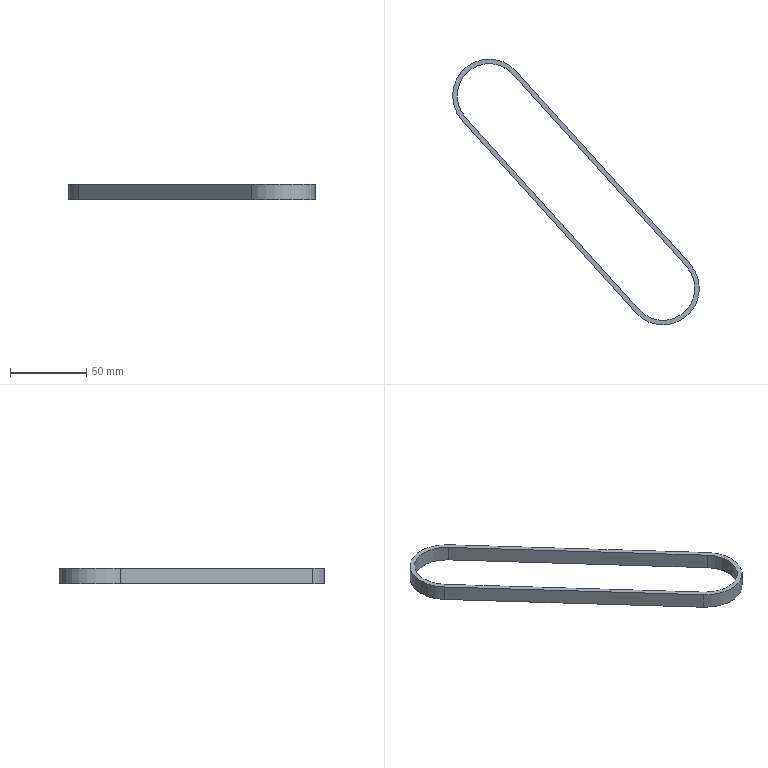Part | STEP file | 1 solid | 12 faces | box 161.812 x 174.281 x 10 mm | volume 14441 mm3 | plane 6 | cylinder 6 | commonest cylinder face diameters 42 x3 48 x3
STEP:
#1=CARTESIAN_POINT('',(0.,0.,0.));
#2=DIRECTION('',(0.,0.,1.));
#3=DIRECTION('',(1.,0.,0.));
#4=AXIS2_PLACEMENT_3D('',#1,#2,#3);
#5=CARTESIAN_POINT('',(15.599,14.059,-2.));
#6=VERTEX_POINT('',#5);
#7=CARTESIAN_POINT('',(-98.213,140.34,-2.));
#8=VERTEX_POINT('',#7);
#9=CARTESIAN_POINT('',(15.599,14.059,-2.));
#10=DIRECTION('',(-0.6695,0.7428,0.));
#11=VECTOR('',#10,1.);
#12=LINE('',#9,#11);
#13=CARTESIAN_POINT('',(15.599,14.059,-12.));
#14=DIRECTION('',(0.7428,0.6695,0.));
#15=DIRECTION('',(0.,0.,-1.));
#16=AXIS2_PLACEMENT_3D('',#13,#14,#15);
#17=PLANE('',#16);
#18=CARTESIAN_POINT('',(-10.,0.));
#19=DIRECTION('',(0.,1.));
#20=VECTOR('',#19,1.);
#21=LINE('',#18,#20);
#22=(GEOMETRIC_REPRESENTATION_CONTEXT(2)PARAMETRIC_REPRESENTATION_CONTEXT()REPRESENTATION_CONTEXT('',''));
#23=DEFINITIONAL_REPRESENTATION('',(#21),#22);
#24=PCURVE('',#17,#23);
#25=CARTESIAN_POINT('',(0.,0.,-2.));
#26=DIRECTION('',(0.,0.,1.));
#27=DIRECTION('',(1.,0.,0.));
#28=AXIS2_PLACEMENT_3D('',#25,#26,#27);
#29=PLANE('',#28);
#30=CARTESIAN_POINT('',(15.599,14.059));
#31=DIRECTION('',(-0.6695,0.7428));
#32=VECTOR('',#31,1.);
#33=LINE('',#30,#32);
#34=(GEOMETRIC_REPRESENTATION_CONTEXT(2)PARAMETRIC_REPRESENTATION_CONTEXT()REPRESENTATION_CONTEXT('',''));
#35=DEFINITIONAL_REPRESENTATION('',(#33),#34);
#36=PCURVE('',#29,#35);
#37=SURFACE_CURVE('',#12,(#24,#36),.PCURVE_S1.);
#38=EDGE_CURVE('',#6,#8,#37,.T.);
#39=ORIENTED_EDGE('',*,*,#38,.T.);
#40=CARTESIAN_POINT('',(-98.213,140.34,-12.));
#41=VERTEX_POINT('',#40);
#42=CARTESIAN_POINT('',(-98.213,140.34,-12.));
#43=DIRECTION('',(0.,0.,1.));
#44=VECTOR('',#43,1.);
#45=LINE('',#42,#44);
#46=CARTESIAN_POINT('',(0.,170.));
#47=DIRECTION('',(-1.,0.));
#48=VECTOR('',#47,1.);
#49=LINE('',#46,#48);
#50=(GEOMETRIC_REPRESENTATION_CONTEXT(2)PARAMETRIC_REPRESENTATION_CONTEXT()REPRESENTATION_CONTEXT('',''));
#51=DEFINITIONAL_REPRESENTATION('',(#49),#50);
#52=PCURVE('',#17,#51);
#53=CARTESIAN_POINT('',(-113.812,126.281,-12.));
#54=DIRECTION('',(0.,0.,1.));
#55=DIRECTION('',(1.,0.,0.));
#56=AXIS2_PLACEMENT_3D('',#53,#54,#55);
#57=CYLINDRICAL_SURFACE('',#56,21.);
#58=CARTESIAN_POINT('',(0.7335,0.));
#59=DIRECTION('',(0.,1.));
#60=VECTOR('',#59,1.);
#61=LINE('',#58,#60);
#62=(GEOMETRIC_REPRESENTATION_CONTEXT(2)PARAMETRIC_REPRESENTATION_CONTEXT()REPRESENTATION_CONTEXT('',''));
#63=DEFINITIONAL_REPRESENTATION('',(#61),#62);
#64=PCURVE('',#57,#63);
#65=SURFACE_CURVE('',#45,(#52,#64),.PCURVE_S1.);
#66=EDGE_CURVE('',#41,#8,#65,.T.);
#67=ORIENTED_EDGE('',*,*,#66,.F.);
#68=CARTESIAN_POINT('',(15.599,14.059,-12.));
#69=VERTEX_POINT('',#68);
#70=CARTESIAN_POINT('',(15.599,14.059,-12.));
#71=DIRECTION('',(-0.6695,0.7428,0.));
#72=VECTOR('',#71,1.);
#73=LINE('',#70,#72);
#74=CARTESIAN_POINT('',(0.,0.));
#75=DIRECTION('',(0.,1.));
#76=VECTOR('',#75,1.);
#77=LINE('',#74,#76);
#78=(GEOMETRIC_REPRESENTATION_CONTEXT(2)PARAMETRIC_REPRESENTATION_CONTEXT()REPRESENTATION_CONTEXT('',''));
#79=DEFINITIONAL_REPRESENTATION('',(#77),#78);
#80=PCURVE('',#17,#79);
#81=CARTESIAN_POINT('',(0.,0.,-12.));
#82=DIRECTION('',(0.,0.,1.));
#83=DIRECTION('',(1.,0.,0.));
#84=AXIS2_PLACEMENT_3D('',#81,#82,#83);
#85=PLANE('',#84);
#86=CARTESIAN_POINT('',(15.599,14.059));
#87=DIRECTION('',(-0.6695,0.7428));
#88=VECTOR('',#87,1.);
#89=LINE('',#86,#88);
#90=(GEOMETRIC_REPRESENTATION_CONTEXT(2)PARAMETRIC_REPRESENTATION_CONTEXT()REPRESENTATION_CONTEXT('',''));
#91=DEFINITIONAL_REPRESENTATION('',(#89),#90);
#92=PCURVE('',#85,#91);
#93=SURFACE_CURVE('',#73,(#80,#92),.PCURVE_S1.);
#94=EDGE_CURVE('',#69,#41,#93,.T.);
#95=ORIENTED_EDGE('',*,*,#94,.F.);
#96=CARTESIAN_POINT('',(15.599,14.059,-12.));
#97=DIRECTION('',(0.,0.,1.));
#98=VECTOR('',#97,1.);
#99=LINE('',#96,#98);
#100=CARTESIAN_POINT('',(0.,0.));
#101=DIRECTION('',(-1.,0.));
#102=VECTOR('',#101,1.);
#103=LINE('',#100,#102);
#104=(GEOMETRIC_REPRESENTATION_CONTEXT(2)PARAMETRIC_REPRESENTATION_CONTEXT()REPRESENTATION_CONTEXT('',''));
#105=DEFINITIONAL_REPRESENTATION('',(#103),#104);
#106=PCURVE('',#17,#105);
#107=CARTESIAN_POINT('',(0.,0.,-12.));
#108=DIRECTION('',(0.,0.,1.));
#109=DIRECTION('',(1.,0.,0.));
#110=AXIS2_PLACEMENT_3D('',#107,#108,#109);
#111=CYLINDRICAL_SURFACE('',#110,21.);
#112=CARTESIAN_POINT('',(0.7335,0.));
#113=DIRECTION('',(0.,1.));
#114=VECTOR('',#113,1.);
#115=LINE('',#112,#114);
#116=(GEOMETRIC_REPRESENTATION_CONTEXT(2)PARAMETRIC_REPRESENTATION_CONTEXT()REPRESENTATION_CONTEXT('',''));
#117=DEFINITIONAL_REPRESENTATION('',(#115),#116);
#118=PCURVE('',#111,#117);
#119=SURFACE_CURVE('',#99,(#106,#118),.PCURVE_S1.);
#120=EDGE_CURVE('',#69,#6,#119,.T.);
#121=ORIENTED_EDGE('',*,*,#120,.T.);
#122=EDGE_LOOP('',(#39,#67,#95,#121));
#123=FACE_BOUND('',#122,.T.);
#124=ADVANCED_FACE('',(#123),#17,.F.);
#125=ORIENTED_EDGE('',*,*,#66,.F.);
#126=CARTESIAN_POINT('',(-129.411,112.222,-12.));
#127=VERTEX_POINT('',#126);
#128=CARTESIAN_POINT('',(-113.812,126.281,-12.));
#129=DIRECTION('',(0.,0.,1.));
#130=DIRECTION('',(1.,0.,0.));
#131=AXIS2_PLACEMENT_3D('',#128,#129,#130);
#132=CIRCLE('',#131,21.);
#133=CARTESIAN_POINT('',(0.,0.));
#134=DIRECTION('',(1.,0.));
#135=VECTOR('',#134,1.);
#136=LINE('',#133,#135);
#137=(GEOMETRIC_REPRESENTATION_CONTEXT(2)PARAMETRIC_REPRESENTATION_CONTEXT()REPRESENTATION_CONTEXT('',''));
#138=DEFINITIONAL_REPRESENTATION('',(#136),#137);
#139=PCURVE('',#57,#138);
#140=CARTESIAN_POINT('',(-113.812,126.281));
#141=DIRECTION('',(1.,0.));
#142=AXIS2_PLACEMENT_2D('',#140,#141);
#143=CIRCLE('',#142,21.);
#144=(GEOMETRIC_REPRESENTATION_CONTEXT(2)PARAMETRIC_REPRESENTATION_CONTEXT()REPRESENTATION_CONTEXT('',''));
#145=DEFINITIONAL_REPRESENTATION('',(#143),#144);
#146=PCURVE('',#85,#145);
#147=SURFACE_CURVE('',#132,(#139,#146),.PCURVE_S1.);
#148=EDGE_CURVE('',#41,#127,#147,.T.);
#149=ORIENTED_EDGE('',*,*,#148,.T.);
#150=CARTESIAN_POINT('',(-129.411,112.222,-2.));
#151=VERTEX_POINT('',#150);
#152=CARTESIAN_POINT('',(-129.411,112.222,-12.));
#153=DIRECTION('',(0.,0.,1.));
#154=VECTOR('',#153,1.);
#155=LINE('',#152,#154);
#156=CARTESIAN_POINT('',(3.875,0.));
#157=DIRECTION('',(0.,1.));
#158=VECTOR('',#157,1.);
#159=LINE('',#156,#158);
#160=(GEOMETRIC_REPRESENTATION_CONTEXT(2)PARAMETRIC_REPRESENTATION_CONTEXT()REPRESENTATION_CONTEXT('',''));
#161=DEFINITIONAL_REPRESENTATION('',(#159),#160);
#162=PCURVE('',#57,#161);
#163=CARTESIAN_POINT('',(-15.599,-14.059,-12.));
#164=DIRECTION('',(-0.7428,-0.6695,0.));
#165=DIRECTION('',(-0.6695,0.7428,0.));
#166=AXIS2_PLACEMENT_3D('',#163,#164,#165);
#167=PLANE('',#166);
#168=CARTESIAN_POINT('',(170.,0.));
#169=DIRECTION('',(0.,-1.));
#170=VECTOR('',#169,1.);
#171=LINE('',#168,#170);
#172=(GEOMETRIC_REPRESENTATION_CONTEXT(2)PARAMETRIC_REPRESENTATION_CONTEXT()REPRESENTATION_CONTEXT('',''));
#173=DEFINITIONAL_REPRESENTATION('',(#171),#172);
#174=PCURVE('',#167,#173);
#175=SURFACE_CURVE('',#155,(#162,#174),.PCURVE_S1.);
#176=EDGE_CURVE('',#127,#151,#175,.T.);
#177=ORIENTED_EDGE('',*,*,#176,.T.);
#178=CARTESIAN_POINT('',(-113.812,126.281,-2.));
#179=DIRECTION('',(0.,0.,1.));
#180=DIRECTION('',(1.,0.,0.));
#181=AXIS2_PLACEMENT_3D('',#178,#179,#180);
#182=CIRCLE('',#181,21.);
#183=CARTESIAN_POINT('',(0.,10.));
#184=DIRECTION('',(1.,0.));
#185=VECTOR('',#184,1.);
#186=LINE('',#183,#185);
#187=(GEOMETRIC_REPRESENTATION_CONTEXT(2)PARAMETRIC_REPRESENTATION_CONTEXT()REPRESENTATION_CONTEXT('',''));
#188=DEFINITIONAL_REPRESENTATION('',(#186),#187);
#189=PCURVE('',#57,#188);
#190=CARTESIAN_POINT('',(-113.812,126.281));
#191=DIRECTION('',(1.,0.));
#192=AXIS2_PLACEMENT_2D('',#190,#191);
#193=CIRCLE('',#192,21.);
#194=(GEOMETRIC_REPRESENTATION_CONTEXT(2)PARAMETRIC_REPRESENTATION_CONTEXT()REPRESENTATION_CONTEXT('',''));
#195=DEFINITIONAL_REPRESENTATION('',(#193),#194);
#196=PCURVE('',#29,#195);
#197=SURFACE_CURVE('',#182,(#189,#196),.PCURVE_S1.);
#198=EDGE_CURVE('',#8,#151,#197,.T.);
#199=ORIENTED_EDGE('',*,*,#198,.F.);
#200=EDGE_LOOP('',(#125,#149,#177,#199));
#201=FACE_BOUND('',#200,.F.);
#202=ADVANCED_FACE('',(#201),#57,.F.);
#203=CARTESIAN_POINT('',(-15.599,-14.059,-2.));
#204=VERTEX_POINT('',#203);
#205=CARTESIAN_POINT('',(-15.599,-14.059,-2.));
#206=DIRECTION('',(0.6695,-0.7428,0.));
#207=VECTOR('',#206,1.);
#208=LINE('',#205,#207);
#209=CARTESIAN_POINT('',(0.,-10.));
#210=DIRECTION('',(-1.,0.));
#211=VECTOR('',#210,1.);
#212=LINE('',#209,#211);
#213=(GEOMETRIC_REPRESENTATION_CONTEXT(2)PARAMETRIC_REPRESENTATION_CONTEXT()REPRESENTATION_CONTEXT('',''));
#214=DEFINITIONAL_REPRESENTATION('',(#212),#213);
#215=PCURVE('',#167,#214);
#216=CARTESIAN_POINT('',(-15.599,-14.059));
#217=DIRECTION('',(0.6695,-0.7428));
#218=VECTOR('',#217,1.);
#219=LINE('',#216,#218);
#220=(GEOMETRIC_REPRESENTATION_CONTEXT(2)PARAMETRIC_REPRESENTATION_CONTEXT()REPRESENTATION_CONTEXT('',''));
#221=DEFINITIONAL_REPRESENTATION('',(#219),#220);
#222=PCURVE('',#29,#221);
#223=SURFACE_CURVE('',#208,(#215,#222),.PCURVE_S1.);
#224=EDGE_CURVE('',#151,#204,#223,.T.);
#225=ORIENTED_EDGE('',*,*,#224,.T.);
#226=CARTESIAN_POINT('',(-15.599,-14.059,-12.));
#227=VERTEX_POINT('',#226);
#228=CARTESIAN_POINT('',(-15.599,-14.059,-12.));
#229=DIRECTION('',(0.,0.,1.));
#230=VECTOR('',#229,1.);
#231=LINE('',#228,#230);
#232=CARTESIAN_POINT('',(0.,0.));
#233=DIRECTION('',(0.,-1.));
#234=VECTOR('',#233,1.);
#235=LINE('',#232,#234);
#236=(GEOMETRIC_REPRESENTATION_CONTEXT(2)PARAMETRIC_REPRESENTATION_CONTEXT()REPRESENTATION_CONTEXT('',''));
#237=DEFINITIONAL_REPRESENTATION('',(#235),#236);
#238=PCURVE('',#167,#237);
#239=CARTESIAN_POINT('',(0.,0.,-12.));
#240=DIRECTION('',(0.,0.,1.));
#241=DIRECTION('',(1.,0.,0.));
#242=AXIS2_PLACEMENT_3D('',#239,#240,#241);
#243=CYLINDRICAL_SURFACE('',#242,21.);
#244=CARTESIAN_POINT('',(3.875,0.));
#245=DIRECTION('',(0.,1.));
#246=VECTOR('',#245,1.);
#247=LINE('',#244,#246);
#248=(GEOMETRIC_REPRESENTATION_CONTEXT(2)PARAMETRIC_REPRESENTATION_CONTEXT()REPRESENTATION_CONTEXT('',''));
#249=DEFINITIONAL_REPRESENTATION('',(#247),#248);
#250=PCURVE('',#243,#249);
#251=SURFACE_CURVE('',#231,(#238,#250),.PCURVE_S1.);
#252=EDGE_CURVE('',#227,#204,#251,.T.);
#253=ORIENTED_EDGE('',*,*,#252,.F.);
#254=CARTESIAN_POINT('',(-15.599,-14.059,-12.));
#255=DIRECTION('',(0.6695,-0.7428,0.));
#256=VECTOR('',#255,1.);
#257=LINE('',#254,#256);
#258=CARTESIAN_POINT('',(0.,0.));
#259=DIRECTION('',(-1.,0.));
#260=VECTOR('',#259,1.);
#261=LINE('',#258,#260);
#262=(GEOMETRIC_REPRESENTATION_CONTEXT(2)PARAMETRIC_REPRESENTATION_CONTEXT()REPRESENTATION_CONTEXT('',''));
#263=DEFINITIONAL_REPRESENTATION('',(#261),#262);
#264=PCURVE('',#167,#263);
#265=CARTESIAN_POINT('',(-15.599,-14.059));
#266=DIRECTION('',(0.6695,-0.7428));
#267=VECTOR('',#266,1.);
#268=LINE('',#265,#267);
#269=(GEOMETRIC_REPRESENTATION_CONTEXT(2)PARAMETRIC_REPRESENTATION_CONTEXT()REPRESENTATION_CONTEXT('',''));
#270=DEFINITIONAL_REPRESENTATION('',(#268),#269);
#271=PCURVE('',#85,#270);
#272=SURFACE_CURVE('',#257,(#264,#271),.PCURVE_S1.);
#273=EDGE_CURVE('',#127,#227,#272,.T.);
#274=ORIENTED_EDGE('',*,*,#273,.F.);
#275=ORIENTED_EDGE('',*,*,#176,.T.);
#276=EDGE_LOOP('',(#225,#253,#274,#275));
#277=FACE_BOUND('',#276,.T.);
#278=ADVANCED_FACE('',(#277),#167,.F.);
#279=CARTESIAN_POINT('',(21.,0.,-2.));
#280=VERTEX_POINT('',#279);
#281=CARTESIAN_POINT('',(0.,0.,-2.));
#282=DIRECTION('',(0.,0.,1.));
#283=DIRECTION('',(1.,0.,0.));
#284=AXIS2_PLACEMENT_3D('',#281,#282,#283);
#285=CIRCLE('',#284,21.);
#286=CARTESIAN_POINT('',(0.,10.));
#287=DIRECTION('',(1.,0.));
#288=VECTOR('',#287,1.);
#289=LINE('',#286,#288);
#290=(GEOMETRIC_REPRESENTATION_CONTEXT(2)PARAMETRIC_REPRESENTATION_CONTEXT()REPRESENTATION_CONTEXT('',''));
#291=DEFINITIONAL_REPRESENTATION('',(#289),#290);
#292=PCURVE('',#243,#291);
#293=CARTESIAN_POINT('',(0.,0.));
#294=DIRECTION('',(1.,0.));
#295=AXIS2_PLACEMENT_2D('',#293,#294);
#296=CIRCLE('',#295,21.);
#297=(GEOMETRIC_REPRESENTATION_CONTEXT(2)PARAMETRIC_REPRESENTATION_CONTEXT()REPRESENTATION_CONTEXT('',''));
#298=DEFINITIONAL_REPRESENTATION('',(#296),#297);
#299=PCURVE('',#29,#298);
#300=SURFACE_CURVE('',#285,(#292,#299),.PCURVE_S1.);
#301=EDGE_CURVE('',#204,#280,#300,.T.);
#302=ORIENTED_EDGE('',*,*,#301,.F.);
#303=ORIENTED_EDGE('',*,*,#252,.F.);
#304=CARTESIAN_POINT('',(21.,0.,-12.));
#305=VERTEX_POINT('',#304);
#306=CARTESIAN_POINT('',(0.,0.,-12.));
#307=DIRECTION('',(0.,0.,1.));
#308=DIRECTION('',(1.,0.,0.));
#309=AXIS2_PLACEMENT_3D('',#306,#307,#308);
#310=CIRCLE('',#309,21.);
#311=CARTESIAN_POINT('',(0.,0.));
#312=DIRECTION('',(1.,0.));
#313=VECTOR('',#312,1.);
#314=LINE('',#311,#313);
#315=(GEOMETRIC_REPRESENTATION_CONTEXT(2)PARAMETRIC_REPRESENTATION_CONTEXT()REPRESENTATION_CONTEXT('',''));
#316=DEFINITIONAL_REPRESENTATION('',(#314),#315);
#317=PCURVE('',#243,#316);
#318=CARTESIAN_POINT('',(0.,0.));
#319=DIRECTION('',(1.,0.));
#320=AXIS2_PLACEMENT_2D('',#318,#319);
#321=CIRCLE('',#320,21.);
#322=(GEOMETRIC_REPRESENTATION_CONTEXT(2)PARAMETRIC_REPRESENTATION_CONTEXT()REPRESENTATION_CONTEXT('',''));
#323=DEFINITIONAL_REPRESENTATION('',(#321),#322);
#324=PCURVE('',#85,#323);
#325=SURFACE_CURVE('',#310,(#317,#324),.PCURVE_S1.);
#326=EDGE_CURVE('',#227,#305,#325,.T.);
#327=ORIENTED_EDGE('',*,*,#326,.T.);
#328=CARTESIAN_POINT('',(21.,0.,-12.));
#329=DIRECTION('',(0.,0.,1.));
#330=VECTOR('',#329,1.);
#331=LINE('',#328,#330);
#332=CARTESIAN_POINT('',(6.283,0.));
#333=DIRECTION('',(0.,1.));
#334=VECTOR('',#333,1.);
#335=LINE('',#332,#334);
#336=(GEOMETRIC_REPRESENTATION_CONTEXT(2)PARAMETRIC_REPRESENTATION_CONTEXT()REPRESENTATION_CONTEXT('',''));
#337=DEFINITIONAL_REPRESENTATION('',(#335),#336);
#338=PCURVE('',#243,#337);
#339=CARTESIAN_POINT('',(0.,0.));
#340=DIRECTION('',(0.,1.));
#341=VECTOR('',#340,1.);
#342=LINE('',#339,#341);
#343=(GEOMETRIC_REPRESENTATION_CONTEXT(2)PARAMETRIC_REPRESENTATION_CONTEXT()REPRESENTATION_CONTEXT('',''));
#344=DEFINITIONAL_REPRESENTATION('',(#342),#343);
#345=PCURVE('',#111,#344);
#346=SURFACE_CURVE('',#331,(#338,#345),.PCURVE_S1.);
#347=EDGE_CURVE('',#305,#280,#346,.T.);
#348=ORIENTED_EDGE('',*,*,#347,.T.);
#349=EDGE_LOOP('',(#302,#303,#327,#348));
#350=FACE_BOUND('',#349,.F.);
#351=ADVANCED_FACE('',(#350),#243,.F.);
#352=ORIENTED_EDGE('',*,*,#301,.F.);
#353=ORIENTED_EDGE('',*,*,#224,.F.);
#354=ORIENTED_EDGE('',*,*,#198,.F.);
#355=ORIENTED_EDGE('',*,*,#38,.F.);
#356=CARTESIAN_POINT('',(0.,0.,-2.));
#357=DIRECTION('',(0.,0.,1.));
#358=DIRECTION('',(1.,0.,0.));
#359=AXIS2_PLACEMENT_3D('',#356,#357,#358);
#360=CIRCLE('',#359,21.);
#361=CARTESIAN_POINT('',(0.,0.));
#362=DIRECTION('',(1.,0.));
#363=AXIS2_PLACEMENT_2D('',#361,#362);
#364=CIRCLE('',#363,21.);
#365=(GEOMETRIC_REPRESENTATION_CONTEXT(2)PARAMETRIC_REPRESENTATION_CONTEXT()REPRESENTATION_CONTEXT('',''));
#366=DEFINITIONAL_REPRESENTATION('',(#364),#365);
#367=PCURVE('',#29,#366);
#368=CARTESIAN_POINT('',(0.,10.));
#369=DIRECTION('',(1.,0.));
#370=VECTOR('',#369,1.);
#371=LINE('',#368,#370);
#372=(GEOMETRIC_REPRESENTATION_CONTEXT(2)PARAMETRIC_REPRESENTATION_CONTEXT()REPRESENTATION_CONTEXT('',''));
#373=DEFINITIONAL_REPRESENTATION('',(#371),#372);
#374=PCURVE('',#111,#373);
#375=SURFACE_CURVE('',#360,(#367,#374),.PCURVE_S1.);
#376=EDGE_CURVE('',#280,#6,#375,.T.);
#377=ORIENTED_EDGE('',*,*,#376,.F.);
#378=EDGE_LOOP('',(#352,#353,#354,#355,#377));
#379=FACE_BOUND('',#378,.T.);
#380=CARTESIAN_POINT('',(-17.828,-16.068,-2.));
#381=VERTEX_POINT('',#380);
#382=CARTESIAN_POINT('',(24.,0.,-2.));
#383=VERTEX_POINT('',#382);
#384=CARTESIAN_POINT('',(0.,0.,-2.));
#385=DIRECTION('',(0.,0.,1.));
#386=DIRECTION('',(1.,0.,0.));
#387=AXIS2_PLACEMENT_3D('',#384,#385,#386);
#388=CIRCLE('',#387,24.);
#389=CARTESIAN_POINT('',(0.,0.));
#390=DIRECTION('',(1.,0.));
#391=AXIS2_PLACEMENT_2D('',#389,#390);
#392=CIRCLE('',#391,24.);
#393=(GEOMETRIC_REPRESENTATION_CONTEXT(2)PARAMETRIC_REPRESENTATION_CONTEXT()REPRESENTATION_CONTEXT('',''));
#394=DEFINITIONAL_REPRESENTATION('',(#392),#393);
#395=PCURVE('',#29,#394);
#396=CARTESIAN_POINT('',(0.,0.,-12.));
#397=DIRECTION('',(0.,0.,1.));
#398=DIRECTION('',(1.,0.,0.));
#399=AXIS2_PLACEMENT_3D('',#396,#397,#398);
#400=CYLINDRICAL_SURFACE('',#399,24.);
#401=CARTESIAN_POINT('',(0.,10.));
#402=DIRECTION('',(1.,0.));
#403=VECTOR('',#402,1.);
#404=LINE('',#401,#403);
#405=(GEOMETRIC_REPRESENTATION_CONTEXT(2)PARAMETRIC_REPRESENTATION_CONTEXT()REPRESENTATION_CONTEXT('',''));
#406=DEFINITIONAL_REPRESENTATION('',(#404),#405);
#407=PCURVE('',#400,#406);
#408=SURFACE_CURVE('',#388,(#395,#407),.PCURVE_S1.);
#409=EDGE_CURVE('',#381,#383,#408,.T.);
#410=ORIENTED_EDGE('',*,*,#409,.T.);
#411=CARTESIAN_POINT('',(17.828,16.068,-2.));
#412=VERTEX_POINT('',#411);
#413=CARTESIAN_POINT('',(0.,0.,-2.));
#414=DIRECTION('',(0.,0.,1.));
#415=DIRECTION('',(1.,0.,0.));
#416=AXIS2_PLACEMENT_3D('',#413,#414,#415);
#417=CIRCLE('',#416,24.);
#418=CARTESIAN_POINT('',(0.,0.));
#419=DIRECTION('',(1.,0.));
#420=AXIS2_PLACEMENT_2D('',#418,#419);
#421=CIRCLE('',#420,24.);
#422=(GEOMETRIC_REPRESENTATION_CONTEXT(2)PARAMETRIC_REPRESENTATION_CONTEXT()REPRESENTATION_CONTEXT('',''));
#423=DEFINITIONAL_REPRESENTATION('',(#421),#422);
#424=PCURVE('',#29,#423);
#425=CARTESIAN_POINT('',(0.,0.,-12.));
#426=DIRECTION('',(0.,0.,1.));
#427=DIRECTION('',(1.,0.,0.));
#428=AXIS2_PLACEMENT_3D('',#425,#426,#427);
#429=CYLINDRICAL_SURFACE('',#428,24.);
#430=CARTESIAN_POINT('',(0.,10.));
#431=DIRECTION('',(1.,0.));
#432=VECTOR('',#431,1.);
#433=LINE('',#430,#432);
#434=(GEOMETRIC_REPRESENTATION_CONTEXT(2)PARAMETRIC_REPRESENTATION_CONTEXT()REPRESENTATION_CONTEXT('',''));
#435=DEFINITIONAL_REPRESENTATION('',(#433),#434);
#436=PCURVE('',#429,#435);
#437=SURFACE_CURVE('',#417,(#424,#436),.PCURVE_S1.);
#438=EDGE_CURVE('',#383,#412,#437,.T.);
#439=ORIENTED_EDGE('',*,*,#438,.T.);
#440=CARTESIAN_POINT('',(-95.984,142.348,-2.));
#441=VERTEX_POINT('',#440);
#442=CARTESIAN_POINT('',(17.828,16.068,-2.));
#443=DIRECTION('',(-0.6695,0.7428,0.));
#444=VECTOR('',#443,1.);
#445=LINE('',#442,#444);
#446=CARTESIAN_POINT('',(17.828,16.068));
#447=DIRECTION('',(-0.6695,0.7428));
#448=VECTOR('',#447,1.);
#449=LINE('',#446,#448);
#450=(GEOMETRIC_REPRESENTATION_CONTEXT(2)PARAMETRIC_REPRESENTATION_CONTEXT()REPRESENTATION_CONTEXT('',''));
#451=DEFINITIONAL_REPRESENTATION('',(#449),#450);
#452=PCURVE('',#29,#451);
#453=CARTESIAN_POINT('',(17.828,16.068,-12.));
#454=DIRECTION('',(0.7428,0.6695,0.));
#455=DIRECTION('',(0.,0.,-1.));
#456=AXIS2_PLACEMENT_3D('',#453,#454,#455);
#457=PLANE('',#456);
#458=CARTESIAN_POINT('',(-10.,0.));
#459=DIRECTION('',(0.,1.));
#460=VECTOR('',#459,1.);
#461=LINE('',#458,#460);
#462=(GEOMETRIC_REPRESENTATION_CONTEXT(2)PARAMETRIC_REPRESENTATION_CONTEXT()REPRESENTATION_CONTEXT('',''));
#463=DEFINITIONAL_REPRESENTATION('',(#461),#462);
#464=PCURVE('',#457,#463);
#465=SURFACE_CURVE('',#445,(#452,#464),.PCURVE_S1.);
#466=EDGE_CURVE('',#412,#441,#465,.T.);
#467=ORIENTED_EDGE('',*,*,#466,.T.);
#468=CARTESIAN_POINT('',(-131.64,110.213,-2.));
#469=VERTEX_POINT('',#468);
#470=CARTESIAN_POINT('',(-113.812,126.281,-2.));
#471=DIRECTION('',(0.,0.,1.));
#472=DIRECTION('',(1.,0.,0.));
#473=AXIS2_PLACEMENT_3D('',#470,#471,#472);
#474=CIRCLE('',#473,24.);
#475=CARTESIAN_POINT('',(-113.812,126.281));
#476=DIRECTION('',(1.,0.));
#477=AXIS2_PLACEMENT_2D('',#475,#476);
#478=CIRCLE('',#477,24.);
#479=(GEOMETRIC_REPRESENTATION_CONTEXT(2)PARAMETRIC_REPRESENTATION_CONTEXT()REPRESENTATION_CONTEXT('',''));
#480=DEFINITIONAL_REPRESENTATION('',(#478),#479);
#481=PCURVE('',#29,#480);
#482=CARTESIAN_POINT('',(-113.812,126.281,-12.));
#483=DIRECTION('',(0.,0.,1.));
#484=DIRECTION('',(1.,0.,0.));
#485=AXIS2_PLACEMENT_3D('',#482,#483,#484);
#486=CYLINDRICAL_SURFACE('',#485,24.);
#487=CARTESIAN_POINT('',(0.,10.));
#488=DIRECTION('',(1.,0.));
#489=VECTOR('',#488,1.);
#490=LINE('',#487,#489);
#491=(GEOMETRIC_REPRESENTATION_CONTEXT(2)PARAMETRIC_REPRESENTATION_CONTEXT()REPRESENTATION_CONTEXT('',''));
#492=DEFINITIONAL_REPRESENTATION('',(#490),#491);
#493=PCURVE('',#486,#492);
#494=SURFACE_CURVE('',#474,(#481,#493),.PCURVE_S1.);
#495=EDGE_CURVE('',#441,#469,#494,.T.);
#496=ORIENTED_EDGE('',*,*,#495,.T.);
#497=CARTESIAN_POINT('',(-17.828,-16.068,-2.));
#498=DIRECTION('',(0.6695,-0.7428,0.));
#499=VECTOR('',#498,1.);
#500=LINE('',#497,#499);
#501=CARTESIAN_POINT('',(-17.828,-16.068));
#502=DIRECTION('',(0.6695,-0.7428));
#503=VECTOR('',#502,1.);
#504=LINE('',#501,#503);
#505=(GEOMETRIC_REPRESENTATION_CONTEXT(2)PARAMETRIC_REPRESENTATION_CONTEXT()REPRESENTATION_CONTEXT('',''));
#506=DEFINITIONAL_REPRESENTATION('',(#504),#505);
#507=PCURVE('',#29,#506);
#508=CARTESIAN_POINT('',(-17.828,-16.068,-12.));
#509=DIRECTION('',(-0.7428,-0.6695,0.));
#510=DIRECTION('',(-0.6695,0.7428,0.));
#511=AXIS2_PLACEMENT_3D('',#508,#509,#510);
#512=PLANE('',#511);
#513=CARTESIAN_POINT('',(0.,-10.));
#514=DIRECTION('',(-1.,0.));
#515=VECTOR('',#514,1.);
#516=LINE('',#513,#515);
#517=(GEOMETRIC_REPRESENTATION_CONTEXT(2)PARAMETRIC_REPRESENTATION_CONTEXT()REPRESENTATION_CONTEXT('',''));
#518=DEFINITIONAL_REPRESENTATION('',(#516),#517);
#519=PCURVE('',#512,#518);
#520=SURFACE_CURVE('',#500,(#507,#519),.PCURVE_S1.);
#521=EDGE_CURVE('',#469,#381,#520,.T.);
#522=ORIENTED_EDGE('',*,*,#521,.T.);
#523=EDGE_LOOP('',(#410,#439,#467,#496,#522));
#524=FACE_BOUND('',#523,.T.);
#525=ADVANCED_FACE('',(#379,#524),#29,.T.);
#526=ORIENTED_EDGE('',*,*,#273,.T.);
#527=ORIENTED_EDGE('',*,*,#326,.T.);
#528=CARTESIAN_POINT('',(0.,0.,-12.));
#529=DIRECTION('',(0.,0.,1.));
#530=DIRECTION('',(1.,0.,0.));
#531=AXIS2_PLACEMENT_3D('',#528,#529,#530);
#532=CIRCLE('',#531,21.);
#533=CARTESIAN_POINT('',(0.,0.));
#534=DIRECTION('',(1.,0.));
#535=AXIS2_PLACEMENT_2D('',#533,#534);
#536=CIRCLE('',#535,21.);
#537=(GEOMETRIC_REPRESENTATION_CONTEXT(2)PARAMETRIC_REPRESENTATION_CONTEXT()REPRESENTATION_CONTEXT('',''));
#538=DEFINITIONAL_REPRESENTATION('',(#536),#537);
#539=PCURVE('',#85,#538);
#540=CARTESIAN_POINT('',(0.,0.));
#541=DIRECTION('',(1.,0.));
#542=VECTOR('',#541,1.);
#543=LINE('',#540,#542);
#544=(GEOMETRIC_REPRESENTATION_CONTEXT(2)PARAMETRIC_REPRESENTATION_CONTEXT()REPRESENTATION_CONTEXT('',''));
#545=DEFINITIONAL_REPRESENTATION('',(#543),#544);
#546=PCURVE('',#111,#545);
#547=SURFACE_CURVE('',#532,(#539,#546),.PCURVE_S1.);
#548=EDGE_CURVE('',#305,#69,#547,.T.);
#549=ORIENTED_EDGE('',*,*,#548,.T.);
#550=ORIENTED_EDGE('',*,*,#94,.T.);
#551=ORIENTED_EDGE('',*,*,#148,.T.);
#552=EDGE_LOOP('',(#526,#527,#549,#550,#551));
#553=FACE_BOUND('',#552,.T.);
#554=CARTESIAN_POINT('',(-17.828,-16.068,-12.));
#555=VERTEX_POINT('',#554);
#556=CARTESIAN_POINT('',(24.,0.,-12.));
#557=VERTEX_POINT('',#556);
#558=CARTESIAN_POINT('',(0.,0.,-12.));
#559=DIRECTION('',(0.,0.,1.));
#560=DIRECTION('',(1.,0.,0.));
#561=AXIS2_PLACEMENT_3D('',#558,#559,#560);
#562=CIRCLE('',#561,24.);
#563=CARTESIAN_POINT('',(0.,0.));
#564=DIRECTION('',(1.,0.));
#565=AXIS2_PLACEMENT_2D('',#563,#564);
#566=CIRCLE('',#565,24.);
#567=(GEOMETRIC_REPRESENTATION_CONTEXT(2)PARAMETRIC_REPRESENTATION_CONTEXT()REPRESENTATION_CONTEXT('',''));
#568=DEFINITIONAL_REPRESENTATION('',(#566),#567);
#569=PCURVE('',#85,#568);
#570=CARTESIAN_POINT('',(0.,0.));
#571=DIRECTION('',(1.,0.));
#572=VECTOR('',#571,1.);
#573=LINE('',#570,#572);
#574=(GEOMETRIC_REPRESENTATION_CONTEXT(2)PARAMETRIC_REPRESENTATION_CONTEXT()REPRESENTATION_CONTEXT('',''));
#575=DEFINITIONAL_REPRESENTATION('',(#573),#574);
#576=PCURVE('',#400,#575);
#577=SURFACE_CURVE('',#562,(#569,#576),.PCURVE_S1.);
#578=EDGE_CURVE('',#555,#557,#577,.T.);
#579=ORIENTED_EDGE('',*,*,#578,.F.);
#580=CARTESIAN_POINT('',(-131.64,110.213,-12.));
#581=VERTEX_POINT('',#580);
#582=CARTESIAN_POINT('',(-17.828,-16.068,-12.));
#583=DIRECTION('',(0.6695,-0.7428,0.));
#584=VECTOR('',#583,1.);
#585=LINE('',#582,#584);
#586=CARTESIAN_POINT('',(-17.828,-16.068));
#587=DIRECTION('',(0.6695,-0.7428));
#588=VECTOR('',#587,1.);
#589=LINE('',#586,#588);
#590=(GEOMETRIC_REPRESENTATION_CONTEXT(2)PARAMETRIC_REPRESENTATION_CONTEXT()REPRESENTATION_CONTEXT('',''));
#591=DEFINITIONAL_REPRESENTATION('',(#589),#590);
#592=PCURVE('',#85,#591);
#593=CARTESIAN_POINT('',(0.,0.));
#594=DIRECTION('',(-1.,0.));
#595=VECTOR('',#594,1.);
#596=LINE('',#593,#595);
#597=(GEOMETRIC_REPRESENTATION_CONTEXT(2)PARAMETRIC_REPRESENTATION_CONTEXT()REPRESENTATION_CONTEXT('',''));
#598=DEFINITIONAL_REPRESENTATION('',(#596),#597);
#599=PCURVE('',#512,#598);
#600=SURFACE_CURVE('',#585,(#592,#599),.PCURVE_S1.);
#601=EDGE_CURVE('',#581,#555,#600,.T.);
#602=ORIENTED_EDGE('',*,*,#601,.F.);
#603=CARTESIAN_POINT('',(-95.984,142.348,-12.));
#604=VERTEX_POINT('',#603);
#605=CARTESIAN_POINT('',(-113.812,126.281,-12.));
#606=DIRECTION('',(0.,0.,1.));
#607=DIRECTION('',(1.,0.,0.));
#608=AXIS2_PLACEMENT_3D('',#605,#606,#607);
#609=CIRCLE('',#608,24.);
#610=CARTESIAN_POINT('',(-113.812,126.281));
#611=DIRECTION('',(1.,0.));
#612=AXIS2_PLACEMENT_2D('',#610,#611);
#613=CIRCLE('',#612,24.);
#614=(GEOMETRIC_REPRESENTATION_CONTEXT(2)PARAMETRIC_REPRESENTATION_CONTEXT()REPRESENTATION_CONTEXT('',''));
#615=DEFINITIONAL_REPRESENTATION('',(#613),#614);
#616=PCURVE('',#85,#615);
#617=CARTESIAN_POINT('',(0.,0.));
#618=DIRECTION('',(1.,0.));
#619=VECTOR('',#618,1.);
#620=LINE('',#617,#619);
#621=(GEOMETRIC_REPRESENTATION_CONTEXT(2)PARAMETRIC_REPRESENTATION_CONTEXT()REPRESENTATION_CONTEXT('',''));
#622=DEFINITIONAL_REPRESENTATION('',(#620),#621);
#623=PCURVE('',#486,#622);
#624=SURFACE_CURVE('',#609,(#616,#623),.PCURVE_S1.);
#625=EDGE_CURVE('',#604,#581,#624,.T.);
#626=ORIENTED_EDGE('',*,*,#625,.F.);
#627=CARTESIAN_POINT('',(17.828,16.068,-12.));
#628=VERTEX_POINT('',#627);
#629=CARTESIAN_POINT('',(17.828,16.068,-12.));
#630=DIRECTION('',(-0.6695,0.7428,0.));
#631=VECTOR('',#630,1.);
#632=LINE('',#629,#631);
#633=CARTESIAN_POINT('',(17.828,16.068));
#634=DIRECTION('',(-0.6695,0.7428));
#635=VECTOR('',#634,1.);
#636=LINE('',#633,#635);
#637=(GEOMETRIC_REPRESENTATION_CONTEXT(2)PARAMETRIC_REPRESENTATION_CONTEXT()REPRESENTATION_CONTEXT('',''));
#638=DEFINITIONAL_REPRESENTATION('',(#636),#637);
#639=PCURVE('',#85,#638);
#640=CARTESIAN_POINT('',(0.,0.));
#641=DIRECTION('',(0.,1.));
#642=VECTOR('',#641,1.);
#643=LINE('',#640,#642);
#644=(GEOMETRIC_REPRESENTATION_CONTEXT(2)PARAMETRIC_REPRESENTATION_CONTEXT()REPRESENTATION_CONTEXT('',''));
#645=DEFINITIONAL_REPRESENTATION('',(#643),#644);
#646=PCURVE('',#457,#645);
#647=SURFACE_CURVE('',#632,(#639,#646),.PCURVE_S1.);
#648=EDGE_CURVE('',#628,#604,#647,.T.);
#649=ORIENTED_EDGE('',*,*,#648,.F.);
#650=CARTESIAN_POINT('',(0.,0.,-12.));
#651=DIRECTION('',(0.,0.,1.));
#652=DIRECTION('',(1.,0.,0.));
#653=AXIS2_PLACEMENT_3D('',#650,#651,#652);
#654=CIRCLE('',#653,24.);
#655=CARTESIAN_POINT('',(0.,0.));
#656=DIRECTION('',(1.,0.));
#657=AXIS2_PLACEMENT_2D('',#655,#656);
#658=CIRCLE('',#657,24.);
#659=(GEOMETRIC_REPRESENTATION_CONTEXT(2)PARAMETRIC_REPRESENTATION_CONTEXT()REPRESENTATION_CONTEXT('',''));
#660=DEFINITIONAL_REPRESENTATION('',(#658),#659);
#661=PCURVE('',#85,#660);
#662=CARTESIAN_POINT('',(0.,0.));
#663=DIRECTION('',(1.,0.));
#664=VECTOR('',#663,1.);
#665=LINE('',#662,#664);
#666=(GEOMETRIC_REPRESENTATION_CONTEXT(2)PARAMETRIC_REPRESENTATION_CONTEXT()REPRESENTATION_CONTEXT('',''));
#667=DEFINITIONAL_REPRESENTATION('',(#665),#666);
#668=PCURVE('',#429,#667);
#669=SURFACE_CURVE('',#654,(#661,#668),.PCURVE_S1.);
#670=EDGE_CURVE('',#557,#628,#669,.T.);
#671=ORIENTED_EDGE('',*,*,#670,.F.);
#672=EDGE_LOOP('',(#579,#602,#626,#649,#671));
#673=FACE_BOUND('',#672,.T.);
#674=ADVANCED_FACE('',(#553,#673),#85,.F.);
#675=ORIENTED_EDGE('',*,*,#466,.F.);
#676=CARTESIAN_POINT('',(17.828,16.068,-12.));
#677=DIRECTION('',(0.,0.,1.));
#678=VECTOR('',#677,1.);
#679=LINE('',#676,#678);
#680=CARTESIAN_POINT('',(0.,0.));
#681=DIRECTION('',(-1.,0.));
#682=VECTOR('',#681,1.);
#683=LINE('',#680,#682);
#684=(GEOMETRIC_REPRESENTATION_CONTEXT(2)PARAMETRIC_REPRESENTATION_CONTEXT()REPRESENTATION_CONTEXT('',''));
#685=DEFINITIONAL_REPRESENTATION('',(#683),#684);
#686=PCURVE('',#457,#685);
#687=CARTESIAN_POINT('',(0.7335,0.));
#688=DIRECTION('',(0.,1.));
#689=VECTOR('',#688,1.);
#690=LINE('',#687,#689);
#691=(GEOMETRIC_REPRESENTATION_CONTEXT(2)PARAMETRIC_REPRESENTATION_CONTEXT()REPRESENTATION_CONTEXT('',''));
#692=DEFINITIONAL_REPRESENTATION('',(#690),#691);
#693=PCURVE('',#429,#692);
#694=SURFACE_CURVE('',#679,(#686,#693),.PCURVE_S1.);
#695=EDGE_CURVE('',#628,#412,#694,.T.);
#696=ORIENTED_EDGE('',*,*,#695,.F.);
#697=ORIENTED_EDGE('',*,*,#648,.T.);
#698=CARTESIAN_POINT('',(-95.984,142.348,-12.));
#699=DIRECTION('',(0.,0.,1.));
#700=VECTOR('',#699,1.);
#701=LINE('',#698,#700);
#702=CARTESIAN_POINT('',(0.,170.));
#703=DIRECTION('',(-1.,0.));
#704=VECTOR('',#703,1.);
#705=LINE('',#702,#704);
#706=(GEOMETRIC_REPRESENTATION_CONTEXT(2)PARAMETRIC_REPRESENTATION_CONTEXT()REPRESENTATION_CONTEXT('',''));
#707=DEFINITIONAL_REPRESENTATION('',(#705),#706);
#708=PCURVE('',#457,#707);
#709=CARTESIAN_POINT('',(0.7335,0.));
#710=DIRECTION('',(0.,1.));
#711=VECTOR('',#710,1.);
#712=LINE('',#709,#711);
#713=(GEOMETRIC_REPRESENTATION_CONTEXT(2)PARAMETRIC_REPRESENTATION_CONTEXT()REPRESENTATION_CONTEXT('',''));
#714=DEFINITIONAL_REPRESENTATION('',(#712),#713);
#715=PCURVE('',#486,#714);
#716=SURFACE_CURVE('',#701,(#708,#715),.PCURVE_S1.);
#717=EDGE_CURVE('',#604,#441,#716,.T.);
#718=ORIENTED_EDGE('',*,*,#717,.T.);
#719=EDGE_LOOP('',(#675,#696,#697,#718));
#720=FACE_BOUND('',#719,.T.);
#721=ADVANCED_FACE('',(#720),#457,.T.);
#722=ORIENTED_EDGE('',*,*,#495,.F.);
#723=ORIENTED_EDGE('',*,*,#717,.F.);
#724=ORIENTED_EDGE('',*,*,#625,.T.);
#725=CARTESIAN_POINT('',(-131.64,110.213,-12.));
#726=DIRECTION('',(0.,0.,1.));
#727=VECTOR('',#726,1.);
#728=LINE('',#725,#727);
#729=CARTESIAN_POINT('',(3.875,0.));
#730=DIRECTION('',(0.,1.));
#731=VECTOR('',#730,1.);
#732=LINE('',#729,#731);
#733=(GEOMETRIC_REPRESENTATION_CONTEXT(2)PARAMETRIC_REPRESENTATION_CONTEXT()REPRESENTATION_CONTEXT('',''));
#734=DEFINITIONAL_REPRESENTATION('',(#732),#733);
#735=PCURVE('',#486,#734);
#736=CARTESIAN_POINT('',(170.,0.));
#737=DIRECTION('',(0.,-1.));
#738=VECTOR('',#737,1.);
#739=LINE('',#736,#738);
#740=(GEOMETRIC_REPRESENTATION_CONTEXT(2)PARAMETRIC_REPRESENTATION_CONTEXT()REPRESENTATION_CONTEXT('',''));
#741=DEFINITIONAL_REPRESENTATION('',(#739),#740);
#742=PCURVE('',#512,#741);
#743=SURFACE_CURVE('',#728,(#735,#742),.PCURVE_S1.);
#744=EDGE_CURVE('',#581,#469,#743,.T.);
#745=ORIENTED_EDGE('',*,*,#744,.T.);
#746=EDGE_LOOP('',(#722,#723,#724,#745));
#747=FACE_BOUND('',#746,.T.);
#748=ADVANCED_FACE('',(#747),#486,.T.);
#749=ORIENTED_EDGE('',*,*,#521,.F.);
#750=ORIENTED_EDGE('',*,*,#744,.F.);
#751=ORIENTED_EDGE('',*,*,#601,.T.);
#752=CARTESIAN_POINT('',(-17.828,-16.068,-12.));
#753=DIRECTION('',(0.,0.,1.));
#754=VECTOR('',#753,1.);
#755=LINE('',#752,#754);
#756=CARTESIAN_POINT('',(0.,0.));
#757=DIRECTION('',(0.,-1.));
#758=VECTOR('',#757,1.);
#759=LINE('',#756,#758);
#760=(GEOMETRIC_REPRESENTATION_CONTEXT(2)PARAMETRIC_REPRESENTATION_CONTEXT()REPRESENTATION_CONTEXT('',''));
#761=DEFINITIONAL_REPRESENTATION('',(#759),#760);
#762=PCURVE('',#512,#761);
#763=CARTESIAN_POINT('',(3.875,0.));
#764=DIRECTION('',(0.,1.));
#765=VECTOR('',#764,1.);
#766=LINE('',#763,#765);
#767=(GEOMETRIC_REPRESENTATION_CONTEXT(2)PARAMETRIC_REPRESENTATION_CONTEXT()REPRESENTATION_CONTEXT('',''));
#768=DEFINITIONAL_REPRESENTATION('',(#766),#767);
#769=PCURVE('',#400,#768);
#770=SURFACE_CURVE('',#755,(#762,#769),.PCURVE_S1.);
#771=EDGE_CURVE('',#555,#381,#770,.T.);
#772=ORIENTED_EDGE('',*,*,#771,.T.);
#773=EDGE_LOOP('',(#749,#750,#751,#772));
#774=FACE_BOUND('',#773,.T.);
#775=ADVANCED_FACE('',(#774),#512,.T.);
#776=CARTESIAN_POINT('',(24.,0.,-12.));
#777=DIRECTION('',(0.,0.,1.));
#778=VECTOR('',#777,1.);
#779=LINE('',#776,#778);
#780=CARTESIAN_POINT('',(0.,0.));
#781=DIRECTION('',(0.,1.));
#782=VECTOR('',#781,1.);
#783=LINE('',#780,#782);
#784=(GEOMETRIC_REPRESENTATION_CONTEXT(2)PARAMETRIC_REPRESENTATION_CONTEXT()REPRESENTATION_CONTEXT('',''));
#785=DEFINITIONAL_REPRESENTATION('',(#783),#784);
#786=PCURVE('',#429,#785);
#787=CARTESIAN_POINT('',(6.283,0.));
#788=DIRECTION('',(0.,1.));
#789=VECTOR('',#788,1.);
#790=LINE('',#787,#789);
#791=(GEOMETRIC_REPRESENTATION_CONTEXT(2)PARAMETRIC_REPRESENTATION_CONTEXT()REPRESENTATION_CONTEXT('',''));
#792=DEFINITIONAL_REPRESENTATION('',(#790),#791);
#793=PCURVE('',#400,#792);
#794=SURFACE_CURVE('',#779,(#786,#793),.PCURVE_S1.);
#795=EDGE_CURVE('',#557,#383,#794,.T.);
#796=ORIENTED_EDGE('',*,*,#795,.F.);
#797=ORIENTED_EDGE('',*,*,#670,.T.);
#798=ORIENTED_EDGE('',*,*,#695,.T.);
#799=ORIENTED_EDGE('',*,*,#438,.F.);
#800=EDGE_LOOP('',(#796,#797,#798,#799));
#801=FACE_BOUND('',#800,.T.);
#802=ADVANCED_FACE('',(#801),#429,.T.);
#803=ORIENTED_EDGE('',*,*,#578,.T.);
#804=ORIENTED_EDGE('',*,*,#795,.T.);
#805=ORIENTED_EDGE('',*,*,#409,.F.);
#806=ORIENTED_EDGE('',*,*,#771,.F.);
#807=EDGE_LOOP('',(#803,#804,#805,#806));
#808=FACE_BOUND('',#807,.T.);
#809=ADVANCED_FACE('',(#808),#400,.T.);
#810=ORIENTED_EDGE('',*,*,#120,.T.);
#811=ORIENTED_EDGE('',*,*,#376,.F.);
#812=ORIENTED_EDGE('',*,*,#347,.F.);
#813=ORIENTED_EDGE('',*,*,#548,.T.);
#814=EDGE_LOOP('',(#810,#811,#812,#813));
#815=FACE_BOUND('',#814,.F.);
#816=ADVANCED_FACE('',(#815),#111,.F.);
#817=CLOSED_SHELL('',(#124,#202,#278,#351,#525,#674,#721,#748,#775,#802,#809,#816));
#818=MANIFOLD_SOLID_BREP('',#817);
#819=(LENGTH_UNIT()NAMED_UNIT(*)SI_UNIT(.MILLI.,.METRE.));
#820=UNCERTAINTY_MEASURE_WITH_UNIT(LENGTH_MEASURE(0.0000001),#819,'','');
#821=(NAMED_UNIT(*)PLANE_ANGLE_UNIT()SI_UNIT($,.RADIAN.));
#822=(NAMED_UNIT(*)SI_UNIT($,.STERADIAN.)SOLID_ANGLE_UNIT());
#823=(GEOMETRIC_REPRESENTATION_CONTEXT(3)GLOBAL_UNCERTAINTY_ASSIGNED_CONTEXT((#820))GLOBAL_UNIT_ASSIGNED_CONTEXT((#819,#821,#822))REPRESENTATION_CONTEXT('',''));
#824=ADVANCED_BREP_SHAPE_REPRESENTATION('',(#4,#818),#823);